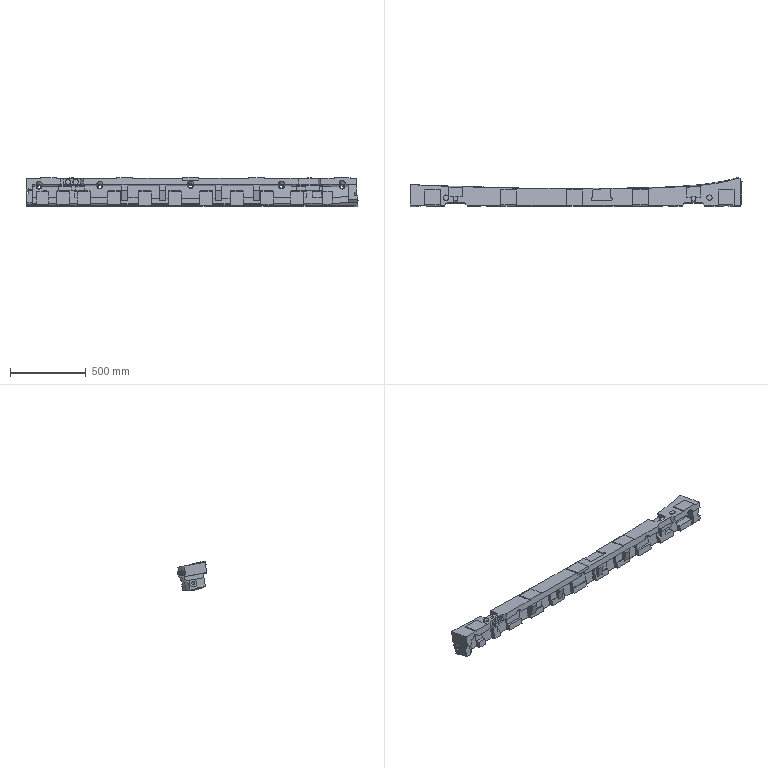Part | NX | features solid 2 | 1 solid | 314 faces | box 2193 x 198.043 x 192.293 mm | volume 26197737 mm3 | plane 194 | spline 81 | cylinder 38 | cone 1 | commonest cylinder face diameters 20 x23 26 x5 40 x5 35 x3 35.4 x1 50 x1